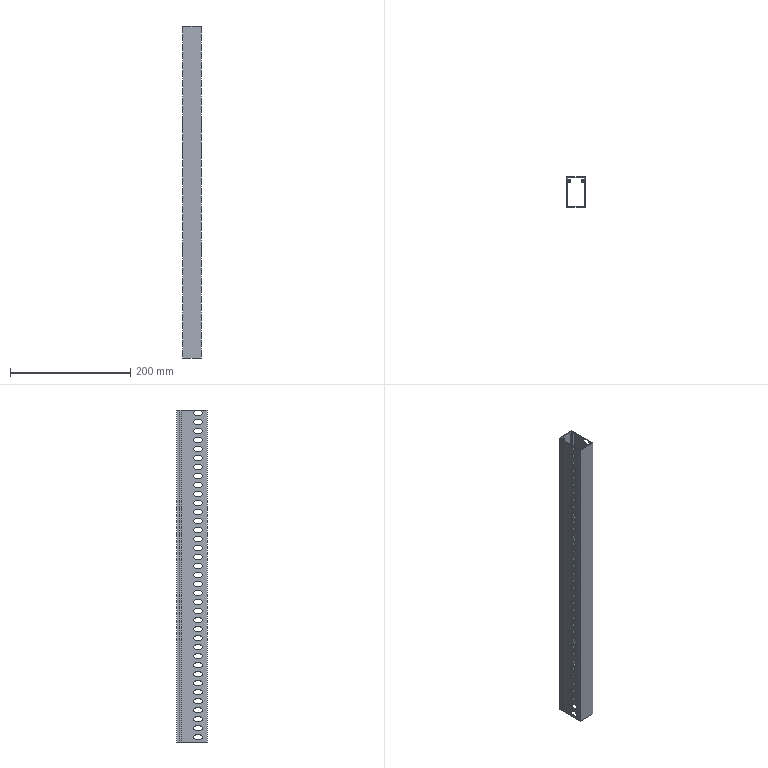Part | SolidWorks | features BaseBody 1 | 1 solid | 322 faces | box 30 x 50 x 553 mm | volume 90056 mm3 | plane 174 | cylinder 148 | commonest cylinder face diameters 8 x148